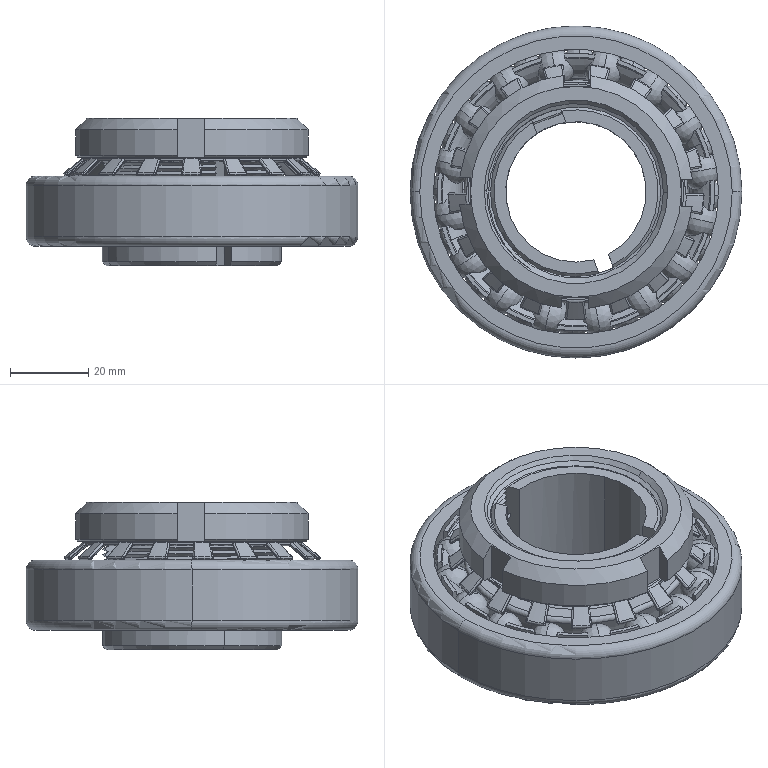Part | SolidWorks | 38 solids | 790 faces | box 85 x 85 x 37.81 mm | volume 92659 mm3 | spline 247 | plane 178 | sphere 128 | torus 123 | cone 58 | cylinder 56 | commonest cylinder face diameters 69 x33 46 x8 0.8 x4 60 x4 36 x3 71 x2